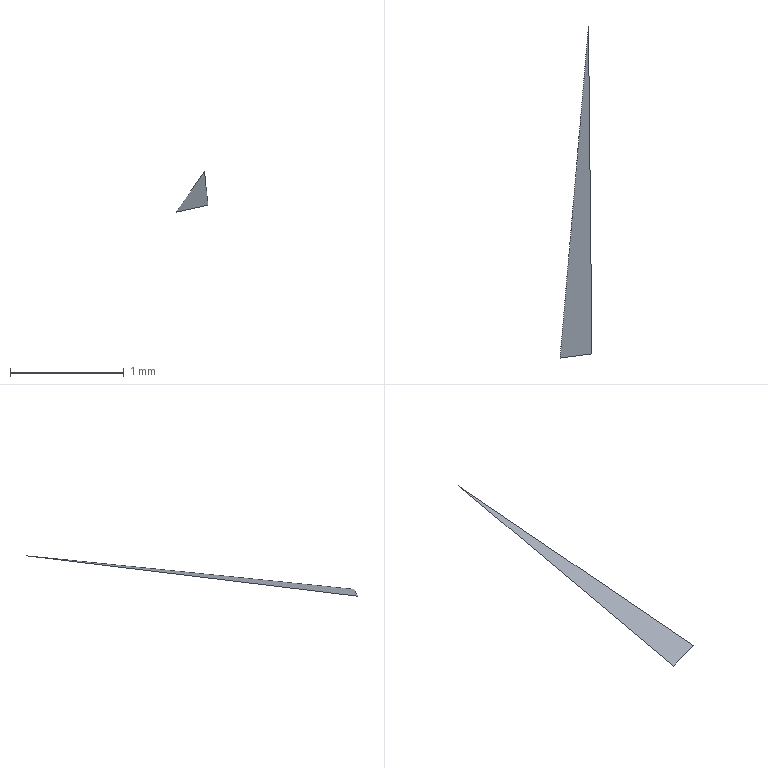Part | NX | features solid 2 | 1 solid | 2 faces | box 0.2806 x 2.95 x 0.36 mm | volume 0.000005266 mm3 | spline 2